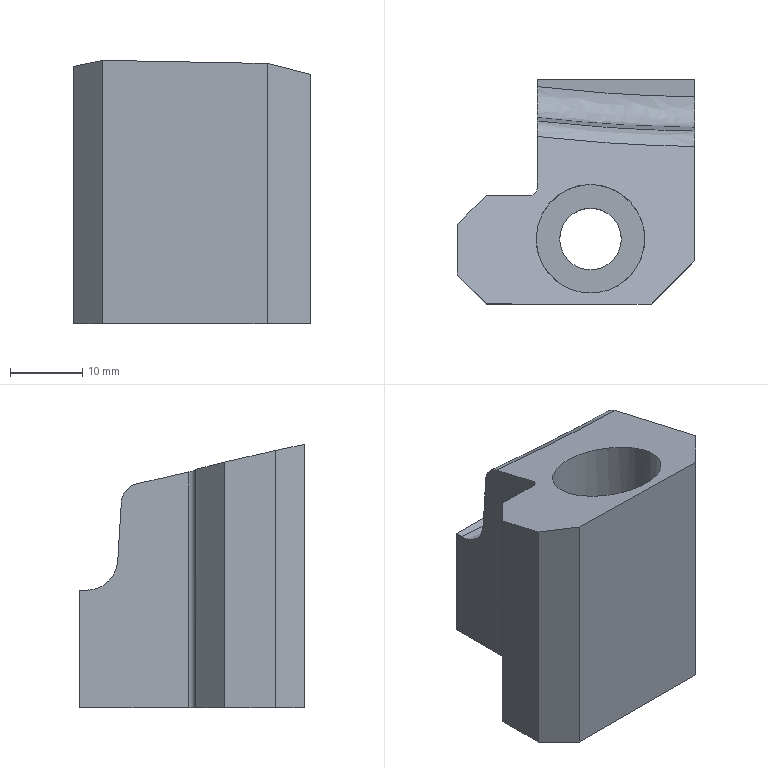Part | STEP file | gslz 2016.10.28-13_id518_x_t | 1 solid | 19 faces | box 32.707 x 31 x 36.324 mm | volume 20957 mm3 | plane 12 | spline 4 | cylinder 3 | commonest cylinder face diameters 2 x1 8.5 x1 15 x1